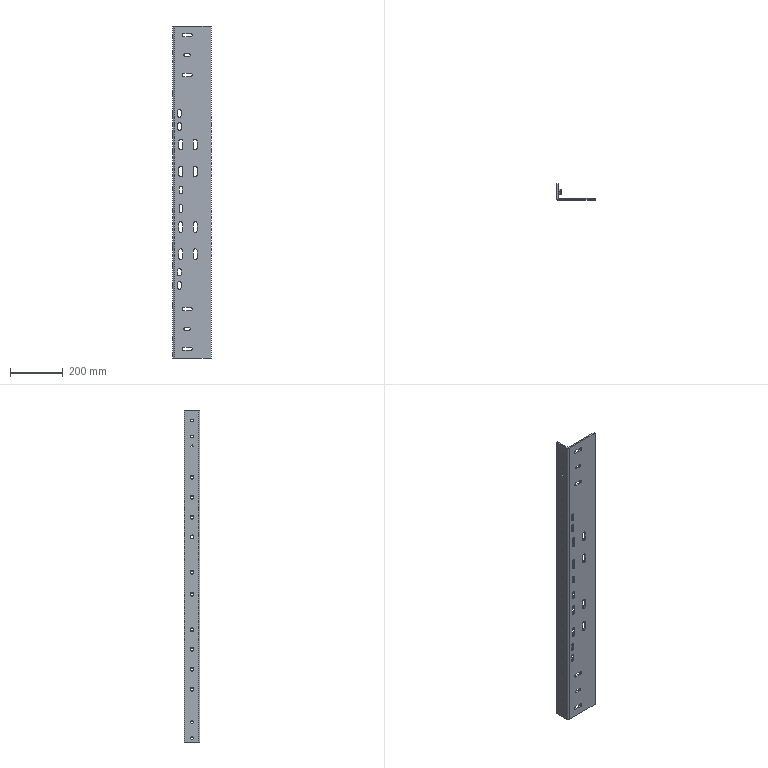Part | 11 solids | 419 faces | box 145 x 60 x 1255 mm | volume 1443722 mm3 | plane 215 | cylinder 144 | cone 60 | commonest cylinder face diameters 13 x26 14 x24 10.647 x20 14.75 x20 15 x20 15.07 x20